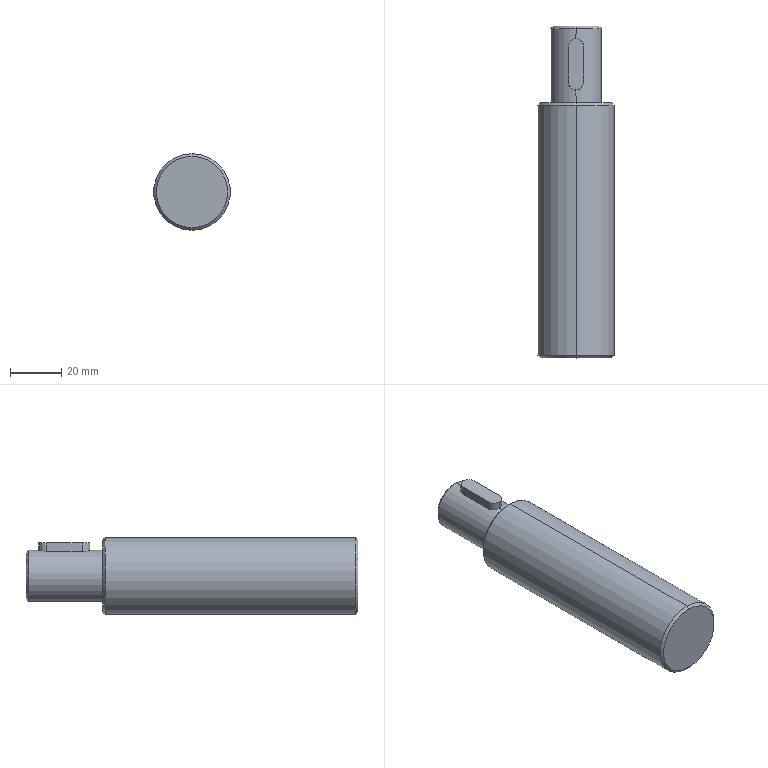Part | SolidWorks | features Chamfer 1, Fillet 1, HoleWzd 1, ICE 1, Revolution 1 | 1 solid | 24 faces | box 30 x 130 x 30 mm | volume 78732 mm3 | cylinder 10 | cone 8 | plane 6 | commonest cylinder face diameters 6 x4 8.5 x2 20 x2 30 x2
STEP:
#1=CARTESIAN_POINT('',(0.,130.,9.));
#2=VERTEX_POINT('',#1);
#3=CARTESIAN_POINT('',(0.,130.,-9.));
#4=VERTEX_POINT('',#3);
#5=CARTESIAN_POINT('',(0.,130.,0.));
#6=DIRECTION('',(0.,1.,0.));
#7=DIRECTION('',(0.,0.,1.));
#8=AXIS2_PLACEMENT_3D('',#5,#6,#7);
#9=CIRCLE('',#8,9.);
#10=EDGE_CURVE('',#2,#4,#9,.T.);
#11=ORIENTED_EDGE('',*,*,#10,.F.);
#12=CARTESIAN_POINT('',(0.,129.,10.));
#13=VERTEX_POINT('',#12);
#14=CARTESIAN_POINT('',(0.,129.,10.));
#15=DIRECTION('',(0.,-0.7071,0.7071));
#16=VECTOR('',#15,1000.);
#17=LINE('',#14,#16);
#18=EDGE_CURVE('',#2,#13,#17,.T.);
#19=ORIENTED_EDGE('',*,*,#18,.T.);
#20=CARTESIAN_POINT('',(0.,129.,-10.));
#21=VERTEX_POINT('',#20);
#22=CARTESIAN_POINT('',(0.,129.,0.));
#23=DIRECTION('',(0.,-1.,0.));
#24=DIRECTION('',(0.,0.,1.));
#25=AXIS2_PLACEMENT_3D('',#22,#23,#24);
#26=CIRCLE('',#25,10.);
#27=EDGE_CURVE('',#21,#13,#26,.T.);
#28=ORIENTED_EDGE('',*,*,#27,.F.);
#29=CARTESIAN_POINT('',(0.,129.,-10.));
#30=DIRECTION('',(0.,-0.7071,-0.7071));
#31=VECTOR('',#30,1000.);
#32=LINE('',#29,#31);
#33=EDGE_CURVE('',#4,#21,#32,.T.);
#34=ORIENTED_EDGE('',*,*,#33,.F.);
#35=EDGE_LOOP('',(#11,#19,#28,#34));
#36=FACE_OUTER_BOUND('',#35,.T.);
#37=CARTESIAN_POINT('',(0.,129.,0.));
#38=DIRECTION('',(0.,-1.,0.));
#39=DIRECTION('',(0.,0.,-1.));
#40=AXIS2_PLACEMENT_3D('',#37,#38,#39);
#41=CONICAL_SURFACE('',#40,10.,0.7854);
#42=ADVANCED_FACE('',(#36),#41,.T.);
#43=CARTESIAN_POINT('',(0.,100.,14.));
#44=VERTEX_POINT('',#43);
#45=CARTESIAN_POINT('',(0.,100.,-14.));
#46=VERTEX_POINT('',#45);
#47=CARTESIAN_POINT('',(0.,100.,0.));
#48=DIRECTION('',(0.,1.,0.));
#49=DIRECTION('',(0.,0.,1.));
#50=AXIS2_PLACEMENT_3D('',#47,#48,#49);
#51=CIRCLE('',#50,14.);
#52=EDGE_CURVE('',#44,#46,#51,.T.);
#53=ORIENTED_EDGE('',*,*,#52,.F.);
#54=CARTESIAN_POINT('',(0.,99.,15.));
#55=VERTEX_POINT('',#54);
#56=CARTESIAN_POINT('',(0.,99.,15.));
#57=DIRECTION('',(0.,-0.7071,0.7071));
#58=VECTOR('',#57,1000.);
#59=LINE('',#56,#58);
#60=EDGE_CURVE('',#44,#55,#59,.T.);
#61=ORIENTED_EDGE('',*,*,#60,.T.);
#62=CARTESIAN_POINT('',(0.,99.,-15.));
#63=VERTEX_POINT('',#62);
#64=CARTESIAN_POINT('',(0.,99.,0.));
#65=DIRECTION('',(0.,-1.,0.));
#66=DIRECTION('',(0.,0.,1.));
#67=AXIS2_PLACEMENT_3D('',#64,#65,#66);
#68=CIRCLE('',#67,15.);
#69=EDGE_CURVE('',#63,#55,#68,.T.);
#70=ORIENTED_EDGE('',*,*,#69,.F.);
#71=CARTESIAN_POINT('',(0.,99.,-15.));
#72=DIRECTION('',(0.,-0.7071,-0.7071));
#73=VECTOR('',#72,1000.);
#74=LINE('',#71,#73);
#75=EDGE_CURVE('',#46,#63,#74,.T.);
#76=ORIENTED_EDGE('',*,*,#75,.F.);
#77=EDGE_LOOP('',(#53,#61,#70,#76));
#78=FACE_OUTER_BOUND('',#77,.T.);
#79=CARTESIAN_POINT('',(0.,99.,0.));
#80=DIRECTION('',(0.,-1.,0.));
#81=DIRECTION('',(0.,0.,-1.));
#82=AXIS2_PLACEMENT_3D('',#79,#80,#81);
#83=CONICAL_SURFACE('',#82,15.,0.7854);
#84=ADVANCED_FACE('',(#78),#83,.T.);
#85=CARTESIAN_POINT('',(0.,0.,-14.));
#86=VERTEX_POINT('',#85);
#87=CARTESIAN_POINT('',(0.,0.,14.));
#88=VERTEX_POINT('',#87);
#89=CARTESIAN_POINT('',(0.,0.,0.));
#90=DIRECTION('',(0.,-1.,0.));
#91=DIRECTION('',(0.,0.,-1.));
#92=AXIS2_PLACEMENT_3D('',#89,#90,#91);
#93=CIRCLE('',#92,14.);
#94=EDGE_CURVE('',#86,#88,#93,.T.);
#95=ORIENTED_EDGE('',*,*,#94,.F.);
#96=CARTESIAN_POINT('',(0.,1.,-15.));
#97=VERTEX_POINT('',#96);
#98=CARTESIAN_POINT('',(0.,0.,-14.));
#99=DIRECTION('',(0.,0.7071,-0.7071));
#100=VECTOR('',#99,1000.);
#101=LINE('',#98,#100);
#102=EDGE_CURVE('',#86,#97,#101,.T.);
#103=ORIENTED_EDGE('',*,*,#102,.T.);
#104=CARTESIAN_POINT('',(0.,1.,15.));
#105=VERTEX_POINT('',#104);
#106=CARTESIAN_POINT('',(0.,1.,0.));
#107=DIRECTION('',(0.,1.,0.));
#108=DIRECTION('',(0.,0.,-1.));
#109=AXIS2_PLACEMENT_3D('',#106,#107,#108);
#110=CIRCLE('',#109,15.);
#111=EDGE_CURVE('',#105,#97,#110,.T.);
#112=ORIENTED_EDGE('',*,*,#111,.F.);
#113=CARTESIAN_POINT('',(0.,0.,14.));
#114=DIRECTION('',(0.,0.7071,0.7071));
#115=VECTOR('',#114,1000.);
#116=LINE('',#113,#115);
#117=EDGE_CURVE('',#88,#105,#116,.T.);
#118=ORIENTED_EDGE('',*,*,#117,.F.);
#119=EDGE_LOOP('',(#95,#103,#112,#118));
#120=FACE_OUTER_BOUND('',#119,.T.);
#121=CARTESIAN_POINT('',(0.,0.,0.));
#122=DIRECTION('',(0.,1.,0.));
#123=DIRECTION('',(0.,0.,1.));
#124=AXIS2_PLACEMENT_3D('',#121,#122,#123);
#125=CONICAL_SURFACE('',#124,14.,0.7854);
#126=ADVANCED_FACE('',(#120),#125,.T.);
#127=CARTESIAN_POINT('',(0.,102.5,-4.25));
#128=VERTEX_POINT('',#127);
#129=CARTESIAN_POINT('',(0.,102.5,4.25));
#130=VERTEX_POINT('',#129);
#131=CARTESIAN_POINT('',(0.,102.5,0.));
#132=DIRECTION('',(0.,1.,0.));
#133=DIRECTION('',(0.,0.,1.));
#134=AXIS2_PLACEMENT_3D('',#131,#132,#133);
#135=CIRCLE('',#134,4.25);
#136=EDGE_CURVE('',#128,#130,#135,.T.);
#137=ORIENTED_EDGE('',*,*,#136,.F.);
#138=CARTESIAN_POINT('',(0.,130.,-4.25));
#139=VERTEX_POINT('',#138);
#140=CARTESIAN_POINT('',(0.,130.,-4.25));
#141=DIRECTION('',(0.,1.,0.));
#142=VECTOR('',#141,1000.);
#143=LINE('',#140,#142);
#144=EDGE_CURVE('',#128,#139,#143,.T.);
#145=ORIENTED_EDGE('',*,*,#144,.T.);
#146=CARTESIAN_POINT('',(0.,130.,4.25));
#147=VERTEX_POINT('',#146);
#148=CARTESIAN_POINT('',(0.,130.,0.));
#149=DIRECTION('',(0.,1.,0.));
#150=DIRECTION('',(0.,0.,1.));
#151=AXIS2_PLACEMENT_3D('',#148,#149,#150);
#152=CIRCLE('',#151,4.25);
#153=EDGE_CURVE('',#139,#147,#152,.T.);
#154=ORIENTED_EDGE('',*,*,#153,.T.);
#155=CARTESIAN_POINT('',(0.,130.,4.25));
#156=DIRECTION('',(0.,1.,0.));
#157=VECTOR('',#156,1000.);
#158=LINE('',#155,#157);
#159=EDGE_CURVE('',#130,#147,#158,.T.);
#160=ORIENTED_EDGE('',*,*,#159,.F.);
#161=EDGE_LOOP('',(#137,#145,#154,#160));
#162=FACE_OUTER_BOUND('',#161,.T.);
#163=CARTESIAN_POINT('',(0.,130.,0.));
#164=DIRECTION('',(0.,1.,0.));
#165=DIRECTION('',(0.,0.,1.));
#166=AXIS2_PLACEMENT_3D('',#163,#164,#165);
#167=CYLINDRICAL_SURFACE('',#166,4.25);
#168=ADVANCED_FACE('',(#162),#167,.F.);
#169=CARTESIAN_POINT('',(0.,99.946,0.));
#170=VERTEX_POINT('',#169);
#171=CARTESIAN_POINT('',(0.,102.5,4.25));
#172=DIRECTION('',(0.,0.515,0.8572));
#173=VECTOR('',#172,1000.);
#174=LINE('',#171,#173);
#175=EDGE_CURVE('',#170,#130,#174,.T.);
#176=ORIENTED_EDGE('',*,*,#175,.F.);
#177=CARTESIAN_POINT('',(0.,102.5,-4.25));
#178=DIRECTION('',(0.,0.515,-0.8572));
#179=VECTOR('',#178,1000.);
#180=LINE('',#177,#179);
#181=EDGE_CURVE('',#170,#128,#180,.T.);
#182=ORIENTED_EDGE('',*,*,#181,.T.);
#183=ORIENTED_EDGE('',*,*,#136,.T.);
#184=EDGE_LOOP('',(#176,#182,#183));
#185=FACE_OUTER_BOUND('',#184,.T.);
#186=CARTESIAN_POINT('',(0.,102.5,0.));
#187=DIRECTION('',(0.,1.,0.));
#188=DIRECTION('',(0.,0.,1.));
#189=AXIS2_PLACEMENT_3D('',#186,#187,#188);
#190=CONICAL_SURFACE('',#189,4.25,1.03);
#191=ADVANCED_FACE('',(#185),#190,.F.);
#192=ORIENTED_EDGE('',*,*,#69,.T.);
#193=CARTESIAN_POINT('',(0.,0.,15.));
#194=DIRECTION('',(0.,-1.,0.));
#195=VECTOR('',#194,1000.);
#196=LINE('',#193,#195);
#197=EDGE_CURVE('',#55,#105,#196,.T.);
#198=ORIENTED_EDGE('',*,*,#197,.T.);
#199=ORIENTED_EDGE('',*,*,#111,.T.);
#200=CARTESIAN_POINT('',(0.,0.,-15.));
#201=DIRECTION('',(0.,-1.,0.));
#202=VECTOR('',#201,1000.);
#203=LINE('',#200,#202);
#204=EDGE_CURVE('',#63,#97,#203,.T.);
#205=ORIENTED_EDGE('',*,*,#204,.F.);
#206=EDGE_LOOP('',(#192,#198,#199,#205));
#207=FACE_OUTER_BOUND('',#206,.T.);
#208=CARTESIAN_POINT('',(0.,0.,0.));
#209=DIRECTION('',(0.,-1.,0.));
#210=DIRECTION('',(0.,0.,-1.));
#211=AXIS2_PLACEMENT_3D('',#208,#209,#210);
#212=CYLINDRICAL_SURFACE('',#211,15.);
#213=ADVANCED_FACE('',(#207),#212,.T.);
#214=ORIENTED_EDGE('',*,*,#27,.T.);
#215=CARTESIAN_POINT('',(0.,125.,10.));
#216=VERTEX_POINT('',#215);
#217=CARTESIAN_POINT('',(0.,0.,10.));
#218=DIRECTION('',(0.,-1.,0.));
#219=VECTOR('',#218,1000.);
#220=LINE('',#217,#219);
#221=EDGE_CURVE('',#13,#216,#220,.T.);
#222=ORIENTED_EDGE('',*,*,#221,.T.);
#223=CARTESIAN_POINT('',(3.,122.,9.539));
#224=VERTEX_POINT('',#223);
#225=CARTESIAN_POINT('',(0.,125.,10.));
#226=CARTESIAN_POINT('',(0.1993,125.,10.));
#227=CARTESIAN_POINT('',(0.3951,124.98,9.994));
#228=CARTESIAN_POINT('',(0.7799,124.903,9.971));
#229=CARTESIAN_POINT('',(0.971,124.845,9.954));
#230=CARTESIAN_POINT('',(1.334,124.694,9.912));
#231=CARTESIAN_POINT('',(1.505,124.602,9.887));
#232=CARTESIAN_POINT('',(1.831,124.385,9.832));
#233=CARTESIAN_POINT('',(1.984,124.259,9.802));
#234=CARTESIAN_POINT('',(2.396,123.847,9.713));
#235=CARTESIAN_POINT('',(2.619,123.514,9.652));
#236=CARTESIAN_POINT('',(2.844,122.974,9.587));
#237=CARTESIAN_POINT('',(2.902,122.784,9.57));
#238=CARTESIAN_POINT('',(2.98,122.396,9.546));
#239=CARTESIAN_POINT('',(3.,122.199,9.539));
#240=CARTESIAN_POINT('',(3.,122.,9.539));
#241=B_SPLINE_CURVE_WITH_KNOTS('',3,(#225,#226,#227,#228,#229,#230,#231,#232,#233,#234,#235,#236,#237,#238,#239,#240),.UNSPECIFIED.,.F.,.F.,(4,2,2,2,2,2,2,4),(0.,0.0005892,0.001178,0.001768,0.002357,0.003535,0.004125,0.004714),.UNSPECIFIED.);
#242=EDGE_CURVE('',#216,#224,#241,.T.);
#243=ORIENTED_EDGE('',*,*,#242,.T.);
#244=CARTESIAN_POINT('',(3.,108.,9.539));
#245=VERTEX_POINT('',#244);
#246=CARTESIAN_POINT('',(3.,0.,9.539));
#247=DIRECTION('',(0.,-1.,0.));
#248=VECTOR('',#247,1000.);
#249=LINE('',#246,#248);
#250=EDGE_CURVE('',#224,#245,#249,.T.);
#251=ORIENTED_EDGE('',*,*,#250,.T.);
#252=CARTESIAN_POINT('',(0.,105.,10.));
#253=VERTEX_POINT('',#252);
#254=CARTESIAN_POINT('',(3.,108.,9.539));
#255=CARTESIAN_POINT('',(3.,107.801,9.539));
#256=CARTESIAN_POINT('',(2.98,107.605,9.546));
#257=CARTESIAN_POINT('',(2.904,107.22,9.569));
#258=CARTESIAN_POINT('',(2.845,107.029,9.587));
#259=CARTESIAN_POINT('',(2.695,106.667,9.63));
#260=CARTESIAN_POINT('',(2.602,106.495,9.656));
#261=CARTESIAN_POINT('',(2.385,106.17,9.712));
#262=CARTESIAN_POINT('',(2.259,106.017,9.742));
#263=CARTESIAN_POINT('',(1.847,105.604,9.832));
#264=CARTESIAN_POINT('',(1.515,105.381,9.891));
#265=CARTESIAN_POINT('',(0.9743,105.156,9.954));
#266=CARTESIAN_POINT('',(0.7845,105.098,9.971));
#267=CARTESIAN_POINT('',(0.3961,105.02,9.994));
#268=CARTESIAN_POINT('',(0.1993,105.,10.));
#269=CARTESIAN_POINT('',(0.,105.,10.));
#270=B_SPLINE_CURVE_WITH_KNOTS('',3,(#254,#255,#256,#257,#258,#259,#260,#261,#262,#263,#264,#265,#266,#267,#268,#269),.UNSPECIFIED.,.F.,.F.,(4,2,2,2,2,2,2,4),(0.,0.0005892,0.001178,0.001768,0.002357,0.003535,0.004125,0.004714),.UNSPECIFIED.);
#271=EDGE_CURVE('',#245,#253,#270,.T.);
#272=ORIENTED_EDGE('',*,*,#271,.T.);
#273=CARTESIAN_POINT('',(0.,100.,10.));
#274=VERTEX_POINT('',#273);
#275=CARTESIAN_POINT('',(0.,0.,10.));
#276=DIRECTION('',(0.,-1.,0.));
#277=VECTOR('',#276,1000.);
#278=LINE('',#275,#277);
#279=EDGE_CURVE('',#253,#274,#278,.T.);
#280=ORIENTED_EDGE('',*,*,#279,.T.);
#281=CARTESIAN_POINT('',(0.,100.,-10.));
#282=VERTEX_POINT('',#281);
#283=CARTESIAN_POINT('',(0.,100.,0.));
#284=DIRECTION('',(0.,-1.,0.));
#285=DIRECTION('',(0.,0.,-1.));
#286=AXIS2_PLACEMENT_3D('',#283,#284,#285);
#287=CIRCLE('',#286,10.);
#288=EDGE_CURVE('',#282,#274,#287,.T.);
#289=ORIENTED_EDGE('',*,*,#288,.F.);
#290=CARTESIAN_POINT('',(0.,0.,-10.));
#291=DIRECTION('',(0.,-1.,0.));
#292=VECTOR('',#291,1000.);
#293=LINE('',#290,#292);
#294=EDGE_CURVE('',#21,#282,#293,.T.);
#295=ORIENTED_EDGE('',*,*,#294,.F.);
#296=EDGE_LOOP('',(#214,#222,#243,#251,#272,#280,#289,#295));
#297=FACE_OUTER_BOUND('',#296,.T.);
#298=CARTESIAN_POINT('',(0.,0.,0.));
#299=DIRECTION('',(0.,-1.,0.));
#300=DIRECTION('',(0.,0.,-1.));
#301=AXIS2_PLACEMENT_3D('',#298,#299,#300);
#302=CYLINDRICAL_SURFACE('',#301,10.);
#303=ADVANCED_FACE('',(#297),#302,.T.);
#304=ORIENTED_EDGE('',*,*,#221,.F.);
#305=CARTESIAN_POINT('',(0.,129.,0.));
#306=DIRECTION('',(0.,-1.,0.));
#307=DIRECTION('',(0.,0.,1.));
#308=AXIS2_PLACEMENT_3D('',#305,#306,#307);
#309=CIRCLE('',#308,10.);
#310=EDGE_CURVE('',#13,#21,#309,.T.);
#311=ORIENTED_EDGE('',*,*,#310,.T.);
#312=ORIENTED_EDGE('',*,*,#294,.T.);
#313=CARTESIAN_POINT('',(0.,100.,0.));
#314=DIRECTION('',(0.,-1.,0.));
#315=DIRECTION('',(0.,0.,-1.));
#316=AXIS2_PLACEMENT_3D('',#313,#314,#315);
#317=CIRCLE('',#316,10.);
#318=EDGE_CURVE('',#274,#282,#317,.T.);
#319=ORIENTED_EDGE('',*,*,#318,.F.);
#320=ORIENTED_EDGE('',*,*,#279,.F.);
#321=CARTESIAN_POINT('',(-3.,108.,9.539));
#322=VERTEX_POINT('',#321);
#323=CARTESIAN_POINT('',(0.,105.,10.));
#324=CARTESIAN_POINT('',(-0.1993,105.,10.));
#325=CARTESIAN_POINT('',(-0.3951,105.02,9.994));
#326=CARTESIAN_POINT('',(-0.7799,105.097,9.971));
#327=CARTESIAN_POINT('',(-0.971,105.155,9.954));
#328=CARTESIAN_POINT('',(-1.334,105.306,9.912));
#329=CARTESIAN_POINT('',(-1.505,105.398,9.887));
#330=CARTESIAN_POINT('',(-1.831,105.615,9.832));
#331=CARTESIAN_POINT('',(-1.984,105.741,9.802));
#332=CARTESIAN_POINT('',(-2.396,106.153,9.713));
#333=CARTESIAN_POINT('',(-2.619,106.486,9.652));
#334=CARTESIAN_POINT('',(-2.844,107.026,9.587));
#335=CARTESIAN_POINT('',(-2.902,107.216,9.57));
#336=CARTESIAN_POINT('',(-2.98,107.604,9.546));
#337=CARTESIAN_POINT('',(-3.,107.801,9.539));
#338=CARTESIAN_POINT('',(-3.,108.,9.539));
#339=B_SPLINE_CURVE_WITH_KNOTS('',3,(#323,#324,#325,#326,#327,#328,#329,#330,#331,#332,#333,#334,#335,#336,#337,#338),.UNSPECIFIED.,.F.,.F.,(4,2,2,2,2,2,2,4),(0.,0.0005892,0.001178,0.001768,0.002357,0.003535,0.004125,0.004714),.UNSPECIFIED.);
#340=EDGE_CURVE('',#253,#322,#339,.T.);
#341=ORIENTED_EDGE('',*,*,#340,.T.);
#342=CARTESIAN_POINT('',(-3.,122.,9.539));
#343=VERTEX_POINT('',#342);
#344=CARTESIAN_POINT('',(-3.,0.,9.539));
#345=DIRECTION('',(0.,1.,0.));
#346=VECTOR('',#345,1000.);
#347=LINE('',#344,#346);
#348=EDGE_CURVE('',#322,#343,#347,.T.);
#349=ORIENTED_EDGE('',*,*,#348,.T.);
#350=CARTESIAN_POINT('',(-3.,122.,9.539));
#351=CARTESIAN_POINT('',(-3.,122.199,9.539));
#352=CARTESIAN_POINT('',(-2.98,122.395,9.546));
#353=CARTESIAN_POINT('',(-2.904,122.78,9.569));
#354=CARTESIAN_POINT('',(-2.845,122.971,9.587));
#355=CARTESIAN_POINT('',(-2.695,123.333,9.63));
#356=CARTESIAN_POINT('',(-2.602,123.505,9.656));
#357=CARTESIAN_POINT('',(-2.385,123.83,9.712));
#358=CARTESIAN_POINT('',(-2.259,123.983,9.742));
#359=CARTESIAN_POINT('',(-1.847,124.396,9.832));
#360=CARTESIAN_POINT('',(-1.515,124.619,9.891));
#361=CARTESIAN_POINT('',(-0.9743,124.844,9.954));
#362=CARTESIAN_POINT('',(-0.7845,124.902,9.971));
#363=CARTESIAN_POINT('',(-0.3961,124.98,9.994));
#364=CARTESIAN_POINT('',(-0.1993,125.,10.));
#365=CARTESIAN_POINT('',(0.,125.,10.));
#366=B_SPLINE_CURVE_WITH_KNOTS('',3,(#350,#351,#352,#353,#354,#355,#356,#357,#358,#359,#360,#361,#362,#363,#364,#365),.UNSPECIFIED.,.F.,.F.,(4,2,2,2,2,2,2,4),(0.,0.0005892,0.001178,0.001768,0.002357,0.003535,0.004125,0.004714),.UNSPECIFIED.);
#367=EDGE_CURVE('',#343,#216,#366,.T.);
#368=ORIENTED_EDGE('',*,*,#367,.T.);
#369=EDGE_LOOP('',(#304,#311,#312,#319,#320,#341,#349,#368));
#370=FACE_OUTER_BOUND('',#369,.T.);
#371=CARTESIAN_POINT('',(0.,0.,0.));
#372=DIRECTION('',(0.,-1.,0.));
#373=DIRECTION('',(0.,0.,-1.));
#374=AXIS2_PLACEMENT_3D('',#371,#372,#373);
#375=CYLINDRICAL_SURFACE('',#374,10.);
#376=ADVANCED_FACE('',(#370),#375,.T.);
#377=CARTESIAN_POINT('',(0.,0.,0.));
#378=DIRECTION('',(0.,-1.,0.));
#379=DIRECTION('',(0.,0.,-1.));
#380=AXIS2_PLACEMENT_3D('',#377,#378,#379);
#381=CIRCLE('',#380,14.);
#382=EDGE_CURVE('',#88,#86,#381,.T.);
#383=ORIENTED_EDGE('',*,*,#382,.T.);
#384=ORIENTED_EDGE('',*,*,#94,.T.);
#385=EDGE_LOOP('',(#383,#384));
#386=FACE_OUTER_BOUND('',#385,.T.);
#387=CARTESIAN_POINT('',(15.,0.,0.));
#388=DIRECTION('',(0.,-1.,0.));
#389=DIRECTION('',(0.,0.,-1.));
#390=AXIS2_PLACEMENT_3D('',#387,#388,#389);
#391=PLANE('',#390);
#392=ADVANCED_FACE('',(#386),#391,.T.);
#393=CARTESIAN_POINT('',(0.,130.,0.));
#394=DIRECTION('',(0.,1.,0.));
#395=DIRECTION('',(0.,0.,1.));
#396=AXIS2_PLACEMENT_3D('',#393,#394,#395);
#397=CIRCLE('',#396,9.);
#398=EDGE_CURVE('',#4,#2,#397,.T.);
#399=ORIENTED_EDGE('',*,*,#398,.T.);
#400=ORIENTED_EDGE('',*,*,#10,.T.);
#401=EDGE_LOOP('',(#399,#400));
#402=FACE_OUTER_BOUND('',#401,.T.);
#403=CARTESIAN_POINT('',(0.,130.,0.));
#404=DIRECTION('',(0.,1.,0.));
#405=DIRECTION('',(0.,0.,1.));
#406=AXIS2_PLACEMENT_3D('',#403,#404,#405);
#407=CIRCLE('',#406,4.25);
#408=EDGE_CURVE('',#147,#139,#407,.T.);
#409=ORIENTED_EDGE('',*,*,#408,.F.);
#410=ORIENTED_EDGE('',*,*,#153,.F.);
#411=EDGE_LOOP('',(#409,#410));
#412=FACE_BOUND('',#411,.T.);
#413=CARTESIAN_POINT('',(0.,130.,0.));
#414=DIRECTION('',(0.,1.,0.));
#415=DIRECTION('',(0.,0.,1.));
#416=AXIS2_PLACEMENT_3D('',#413,#414,#415);
#417=PLANE('',#416);
#418=ADVANCED_FACE('',(#402,#412),#417,.T.);
#419=CARTESIAN_POINT('',(0.,100.,0.));
#420=DIRECTION('',(0.,1.,0.));
#421=DIRECTION('',(0.,0.,1.));
#422=AXIS2_PLACEMENT_3D('',#419,#420,#421);
#423=CIRCLE('',#422,14.);
#424=EDGE_CURVE('',#46,#44,#423,.T.);
#425=ORIENTED_EDGE('',*,*,#424,.T.);
#426=ORIENTED_EDGE('',*,*,#52,.T.);
#427=EDGE_LOOP('',(#425,#426));
#428=FACE_OUTER_BOUND('',#427,.T.);
#429=ORIENTED_EDGE('',*,*,#288,.T.);
#430=ORIENTED_EDGE('',*,*,#318,.T.);
#431=EDGE_LOOP('',(#429,#430));
#432=FACE_BOUND('',#431,.T.);
#433=CARTESIAN_POINT('',(10.,100.,0.));
#434=DIRECTION('',(0.,1.,0.));
#435=DIRECTION('',(0.,0.,1.));
#436=AXIS2_PLACEMENT_3D('',#433,#434,#435);
#437=PLANE('',#436);
#438=ADVANCED_FACE('',(#428,#432),#437,.T.);
#439=ORIENTED_EDGE('',*,*,#197,.F.);
#440=CARTESIAN_POINT('',(0.,99.,0.));
#441=DIRECTION('',(0.,-1.,0.));
#442=DIRECTION('',(0.,0.,1.));
#443=AXIS2_PLACEMENT_3D('',#440,#441,#442);
#444=CIRCLE('',#443,15.);
#445=EDGE_CURVE('',#55,#63,#444,.T.);
#446=ORIENTED_EDGE('',*,*,#445,.T.);
#447=ORIENTED_EDGE('',*,*,#204,.T.);
#448=CARTESIAN_POINT('',(0.,1.,0.));
#449=DIRECTION('',(0.,1.,0.));
#450=DIRECTION('',(0.,0.,-1.));
#451=AXIS2_PLACEMENT_3D('',#448,#449,#450);
#452=CIRCLE('',#451,15.);
#453=EDGE_CURVE('',#97,#105,#452,.T.);
#454=ORIENTED_EDGE('',*,*,#453,.T.);
#455=EDGE_LOOP('',(#439,#446,#447,#454));
#456=FACE_OUTER_BOUND('',#455,.T.);
#457=CARTESIAN_POINT('',(0.,0.,0.));
#458=DIRECTION('',(0.,-1.,0.));
#459=DIRECTION('',(0.,0.,-1.));
#460=AXIS2_PLACEMENT_3D('',#457,#458,#459);
#461=CYLINDRICAL_SURFACE('',#460,15.);
#462=ADVANCED_FACE('',(#456),#461,.T.);
#463=ORIENTED_EDGE('',*,*,#348,.F.);
#464=CARTESIAN_POINT('',(-3.,108.,13.));
#465=VERTEX_POINT('',#464);
#466=CARTESIAN_POINT('',(-3.,108.,13.));
#467=DIRECTION('',(0.,0.,1.));
#468=VECTOR('',#467,1000.);
#469=LINE('',#466,#468);
#470=EDGE_CURVE('',#322,#465,#469,.T.);
#471=ORIENTED_EDGE('',*,*,#470,.T.);
#472=CARTESIAN_POINT('',(-3.,122.,13.));
#473=VERTEX_POINT('',#472);
#474=CARTESIAN_POINT('',(-3.,125.,13.));
#475=DIRECTION('',(0.,-1.,0.));
#476=VECTOR('',#475,1000.);
#477=LINE('',#474,#476);
#478=EDGE_CURVE('',#473,#465,#477,.T.);
#479=ORIENTED_EDGE('',*,*,#478,.F.);
#480=CARTESIAN_POINT('',(-3.,122.,13.));
#481=DIRECTION('',(0.,0.,-1.));
#482=VECTOR('',#481,1000.);
#483=LINE('',#480,#482);
#484=EDGE_CURVE('',#473,#343,#483,.T.);
#485=ORIENTED_EDGE('',*,*,#484,.T.);
#486=EDGE_LOOP('',(#463,#471,#479,#485));
#487=FACE_OUTER_BOUND('',#486,.T.);
#488=CARTESIAN_POINT('',(-3.,125.,13.));
#489=DIRECTION('',(1.,0.,0.));
#490=DIRECTION('',(0.,1.,0.));
#491=AXIS2_PLACEMENT_3D('',#488,#489,#490);
#492=PLANE('',#491);
#493=ADVANCED_FACE('',(#487),#492,.F.);
#494=CARTESIAN_POINT('',(3.,108.,13.));
#495=VERTEX_POINT('',#494);
#496=CARTESIAN_POINT('',(3.,122.,13.));
#497=VERTEX_POINT('',#496);
#498=CARTESIAN_POINT('',(3.,125.,13.));
#499=DIRECTION('',(0.,1.,0.));
#500=VECTOR('',#499,1000.);
#501=LINE('',#498,#500);
#502=EDGE_CURVE('',#495,#497,#501,.T.);
#503=ORIENTED_EDGE('',*,*,#502,.F.);
#504=CARTESIAN_POINT('',(3.,108.,13.));
#505=DIRECTION('',(0.,0.,-1.));
#506=VECTOR('',#505,1000.);
#507=LINE('',#504,#506);
#508=EDGE_CURVE('',#495,#245,#507,.T.);
#509=ORIENTED_EDGE('',*,*,#508,.T.);
#510=ORIENTED_EDGE('',*,*,#250,.F.);
#511=CARTESIAN_POINT('',(3.,122.,13.));
#512=DIRECTION('',(0.,0.,1.));
#513=VECTOR('',#512,1000.);
#514=LINE('',#511,#513);
#515=EDGE_CURVE('',#224,#497,#514,.T.);
#516=ORIENTED_EDGE('',*,*,#515,.T.);
#517=EDGE_LOOP('',(#503,#509,#510,#516));
#518=FACE_OUTER_BOUND('',#517,.T.);
#519=CARTESIAN_POINT('',(3.,125.,13.));
#520=DIRECTION('',(-1.,0.,0.));
#521=DIRECTION('',(0.,-1.,0.));
#522=AXIS2_PLACEMENT_3D('',#519,#520,#521);
#523=PLANE('',#522);
#524=ADVANCED_FACE('',(#518),#523,.F.);
#525=CARTESIAN_POINT('',(0.,105.,13.));
#526=VERTEX_POINT('',#525);
#527=CARTESIAN_POINT('',(0.,108.,13.));
#528=DIRECTION('',(0.,0.,1.));
#529=DIRECTION('',(1.,0.,0.));
#530=AXIS2_PLACEMENT_3D('',#527,#528,#529);
#531=CIRCLE('',#530,3.);
#532=EDGE_CURVE('',#465,#526,#531,.T.);
#533=ORIENTED_EDGE('',*,*,#532,.T.);
#534=CARTESIAN_POINT('',(0.,108.,13.));
#535=DIRECTION('',(0.,0.,1.));
#536=DIRECTION('',(1.,0.,0.));
#537=AXIS2_PLACEMENT_3D('',#534,#535,#536);
#538=CIRCLE('',#537,3.);
#539=EDGE_CURVE('',#526,#495,#538,.T.);
#540=ORIENTED_EDGE('',*,*,#539,.T.);
#541=ORIENTED_EDGE('',*,*,#502,.T.);
#542=CARTESIAN_POINT('',(0.,125.,13.));
#543=VERTEX_POINT('',#542);
#544=CARTESIAN_POINT('',(0.,122.,13.));
#545=DIRECTION('',(0.,0.,1.));
#546=DIRECTION('',(1.,0.,0.));
#547=AXIS2_PLACEMENT_3D('',#544,#545,#546);
#548=CIRCLE('',#547,3.);
#549=EDGE_CURVE('',#497,#543,#548,.T.);
#550=ORIENTED_EDGE('',*,*,#549,.T.);
#551=CARTESIAN_POINT('',(0.,122.,13.));
#552=DIRECTION('',(0.,0.,1.));
#553=DIRECTION('',(1.,0.,0.));
#554=AXIS2_PLACEMENT_3D('',#551,#552,#553);
#555=CIRCLE('',#554,3.);
#556=EDGE_CURVE('',#543,#473,#555,.T.);
#557=ORIENTED_EDGE('',*,*,#556,.T.);
#558=ORIENTED_EDGE('',*,*,#478,.T.);
#559=EDGE_LOOP('',(#533,#540,#541,#550,#557,#558));
#560=FACE_OUTER_BOUND('',#559,.T.);
#561=CARTESIAN_POINT('',(0.,0.,13.));
#562=DIRECTION('',(0.,0.,1.));
#563=DIRECTION('',(1.,0.,0.));
#564=AXIS2_PLACEMENT_3D('',#561,#562,#563);
#565=PLANE('',#564);
#566=ADVANCED_FACE('',(#560),#565,.T.);
#567=CARTESIAN_POINT('',(0.,105.,13.));
#568=DIRECTION('',(0.,0.,-1.));
#569=VECTOR('',#568,1000.);
#570=LINE('',#567,#569);
#571=EDGE_CURVE('',#526,#253,#570,.T.);
#572=ORIENTED_EDGE('',*,*,#571,.F.);
#573=ORIENTED_EDGE('',*,*,#532,.F.);
#574=ORIENTED_EDGE('',*,*,#470,.F.);
#575=ORIENTED_EDGE('',*,*,#340,.F.);
#576=EDGE_LOOP('',(#572,#573,#574,#575));
#577=FACE_OUTER_BOUND('',#576,.T.);
#578=CARTESIAN_POINT('',(0.,108.,13.));
#579=DIRECTION('',(0.,0.,-1.));
#580=DIRECTION('',(-1.,0.,0.));
#581=AXIS2_PLACEMENT_3D('',#578,#579,#580);
#582=CYLINDRICAL_SURFACE('',#581,3.);
#583=ADVANCED_FACE('',(#577),#582,.T.);
#584=ORIENTED_EDGE('',*,*,#539,.F.);
#585=ORIENTED_EDGE('',*,*,#571,.T.);
#586=ORIENTED_EDGE('',*,*,#271,.F.);
#587=ORIENTED_EDGE('',*,*,#508,.F.);
#588=EDGE_LOOP('',(#584,#585,#586,#587));
#589=FACE_OUTER_BOUND('',#588,.T.);
#590=CARTESIAN_POINT('',(0.,108.,13.));
#591=DIRECTION('',(0.,0.,-1.));
#592=DIRECTION('',(-1.,0.,0.));
#593=AXIS2_PLACEMENT_3D('',#590,#591,#592);
#594=CYLINDRICAL_SURFACE('',#593,3.);
#595=ADVANCED_FACE('',(#589),#594,.T.);
#596=ORIENTED_EDGE('',*,*,#484,.F.);
#597=ORIENTED_EDGE('',*,*,#556,.F.);
#598=CARTESIAN_POINT('',(0.,125.,13.));
#599=DIRECTION('',(0.,0.,1.));
#600=VECTOR('',#599,1000.);
#601=LINE('',#598,#600);
#602=EDGE_CURVE('',#216,#543,#601,.T.);
#603=ORIENTED_EDGE('',*,*,#602,.F.);
#604=ORIENTED_EDGE('',*,*,#367,.F.);
#605=EDGE_LOOP('',(#596,#597,#603,#604));
#606=FACE_OUTER_BOUND('',#605,.T.);
#607=CARTESIAN_POINT('',(0.,122.,13.));
#608=DIRECTION('',(0.,0.,-1.));
#609=DIRECTION('',(-1.,0.,0.));
#610=AXIS2_PLACEMENT_3D('',#607,#608,#609);
#611=CYLINDRICAL_SURFACE('',#610,3.);
#612=ADVANCED_FACE('',(#606),#611,.T.);
#613=ORIENTED_EDGE('',*,*,#549,.F.);
#614=ORIENTED_EDGE('',*,*,#515,.F.);
#615=ORIENTED_EDGE('',*,*,#242,.F.);
#616=ORIENTED_EDGE('',*,*,#602,.T.);
#617=EDGE_LOOP('',(#613,#614,#615,#616));
#618=FACE_OUTER_BOUND('',#617,.T.);
#619=CARTESIAN_POINT('',(0.,122.,13.));
#620=DIRECTION('',(0.,0.,-1.));
#621=DIRECTION('',(-1.,0.,0.));
#622=AXIS2_PLACEMENT_3D('',#619,#620,#621);
#623=CYLINDRICAL_SURFACE('',#622,3.);
#624=ADVANCED_FACE('',(#618),#623,.T.);
#625=ORIENTED_EDGE('',*,*,#181,.F.);
#626=ORIENTED_EDGE('',*,*,#175,.T.);
#627=CARTESIAN_POINT('',(0.,102.5,0.));
#628=DIRECTION('',(0.,1.,0.));
#629=DIRECTION('',(0.,0.,1.));
#630=AXIS2_PLACEMENT_3D('',#627,#628,#629);
#631=CIRCLE('',#630,4.25);
#632=EDGE_CURVE('',#130,#128,#631,.T.);
#633=ORIENTED_EDGE('',*,*,#632,.T.);
#634=EDGE_LOOP('',(#625,#626,#633));
#635=FACE_OUTER_BOUND('',#634,.T.);
#636=CARTESIAN_POINT('',(0.,102.5,0.));
#637=DIRECTION('',(0.,1.,0.));
#638=DIRECTION('',(0.,0.,1.));
#639=AXIS2_PLACEMENT_3D('',#636,#637,#638);
#640=CONICAL_SURFACE('',#639,4.25,1.03);
#641=ADVANCED_FACE('',(#635),#640,.F.);
#642=ORIENTED_EDGE('',*,*,#144,.F.);
#643=ORIENTED_EDGE('',*,*,#632,.F.);
#644=ORIENTED_EDGE('',*,*,#159,.T.);
#645=ORIENTED_EDGE('',*,*,#408,.T.);
#646=EDGE_LOOP('',(#642,#643,#644,#645));
#647=FACE_OUTER_BOUND('',#646,.T.);
#648=CARTESIAN_POINT('',(0.,130.,0.));
#649=DIRECTION('',(0.,1.,0.));
#650=DIRECTION('',(0.,0.,1.));
#651=AXIS2_PLACEMENT_3D('',#648,#649,#650);
#652=CYLINDRICAL_SURFACE('',#651,4.25);
#653=ADVANCED_FACE('',(#647),#652,.F.);
#654=ORIENTED_EDGE('',*,*,#102,.F.);
#655=ORIENTED_EDGE('',*,*,#382,.F.);
#656=ORIENTED_EDGE('',*,*,#117,.T.);
#657=ORIENTED_EDGE('',*,*,#453,.F.);
#658=EDGE_LOOP('',(#654,#655,#656,#657));
#659=FACE_OUTER_BOUND('',#658,.T.);
#660=CARTESIAN_POINT('',(0.,0.,0.));
#661=DIRECTION('',(0.,1.,0.));
#662=DIRECTION('',(0.,0.,1.));
#663=AXIS2_PLACEMENT_3D('',#660,#661,#662);
#664=CONICAL_SURFACE('',#663,14.,0.7854);
#665=ADVANCED_FACE('',(#659),#664,.T.);
#666=ORIENTED_EDGE('',*,*,#60,.F.);
#667=ORIENTED_EDGE('',*,*,#424,.F.);
#668=ORIENTED_EDGE('',*,*,#75,.T.);
#669=ORIENTED_EDGE('',*,*,#445,.F.);
#670=EDGE_LOOP('',(#666,#667,#668,#669));
#671=FACE_OUTER_BOUND('',#670,.T.);
#672=CARTESIAN_POINT('',(0.,99.,0.));
#673=DIRECTION('',(0.,-1.,0.));
#674=DIRECTION('',(0.,0.,-1.));
#675=AXIS2_PLACEMENT_3D('',#672,#673,#674);
#676=CONICAL_SURFACE('',#675,15.,0.7854);
#677=ADVANCED_FACE('',(#671),#676,.T.);
#678=ORIENTED_EDGE('',*,*,#18,.F.);
#679=ORIENTED_EDGE('',*,*,#398,.F.);
#680=ORIENTED_EDGE('',*,*,#33,.T.);
#681=ORIENTED_EDGE('',*,*,#310,.F.);
#682=EDGE_LOOP('',(#678,#679,#680,#681));
#683=FACE_OUTER_BOUND('',#682,.T.);
#684=CARTESIAN_POINT('',(0.,129.,0.));
#685=DIRECTION('',(0.,-1.,0.));
#686=DIRECTION('',(0.,0.,-1.));
#687=AXIS2_PLACEMENT_3D('',#684,#685,#686);
#688=CONICAL_SURFACE('',#687,10.,0.7854);
#689=ADVANCED_FACE('',(#683),#688,.T.);
#690=CLOSED_SHELL('',(#42,#84,#126,#168,#191,#213,#303,#376,#392,#418,#438,#462,#493,#524,#566,#583,#595,#612,#624,#641,#653,#665,#677,#689));
#691=MANIFOLD_SOLID_BREP('',#690);
#692=CARTESIAN_POINT('',(0.,0.,0.));
#693=DIRECTION('',(0.,0.,1.));
#694=DIRECTION('',(1.,0.,0.));
#695=AXIS2_PLACEMENT_3D('',#692,#693,#694);
#696=(LENGTH_UNIT()NAMED_UNIT(*)SI_UNIT(.MILLI.,.METRE.));
#697=UNCERTAINTY_MEASURE_WITH_UNIT(LENGTH_MEASURE(0.00001),#696,'','');
#698=(NAMED_UNIT(*)PLANE_ANGLE_UNIT()SI_UNIT($,.RADIAN.));
#699=(NAMED_UNIT(*)SI_UNIT($,.STERADIAN.)SOLID_ANGLE_UNIT());
#700=(GEOMETRIC_REPRESENTATION_CONTEXT(3)GLOBAL_UNCERTAINTY_ASSIGNED_CONTEXT((#697))GLOBAL_UNIT_ASSIGNED_CONTEXT((#696,#698,#699))REPRESENTATION_CONTEXT('',''));
#701=ADVANCED_BREP_SHAPE_REPRESENTATION('',(#691,#695),#700);